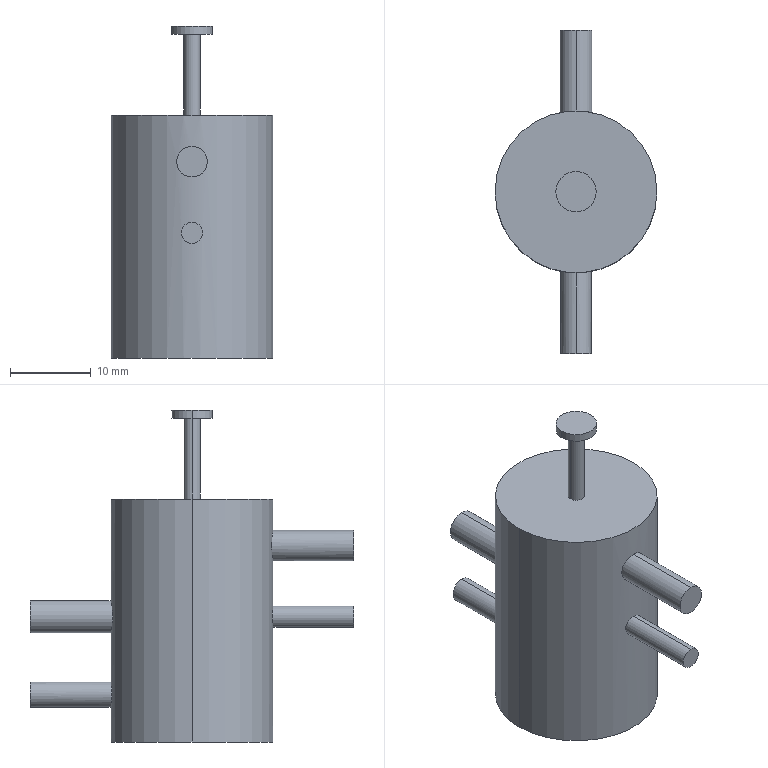Part | SolidWorks | features BaseBody 1 | 1 solid | 22 faces | box 20 x 40 x 41 mm | volume 9841 mm3 | cylinder 14 | plane 8 | commonest cylinder face diameters 2 x2 2.618 x2 3.076 x2 3.768 x2 3.973 x2 5 x2
STEP:
#1=CARTESIAN_POINT('',(0.,-20.,26.133));
#2=VERTEX_POINT('',#1);
#3=CARTESIAN_POINT('',(0.,-20.,22.365));
#4=VERTEX_POINT('',#3);
#5=CARTESIAN_POINT('',(0.,-20.,24.249));
#6=DIRECTION('',(0.,1.,0.));
#7=DIRECTION('',(0.,0.,1.));
#8=AXIS2_PLACEMENT_3D('',#5,#6,#7);
#9=CIRCLE('',#8,1.884);
#10=EDGE_CURVE('',#2,#4,#9,.T.);
#11=ORIENTED_EDGE('',*,*,#10,.T.);
#12=CARTESIAN_POINT('',(0.,-10.,22.365));
#13=VERTEX_POINT('',#12);
#14=CARTESIAN_POINT('',(0.,-20.,22.365));
#15=DIRECTION('',(0.,1.,0.));
#16=VECTOR('',#15,1000.);
#17=LINE('',#14,#16);
#18=EDGE_CURVE('',#4,#13,#17,.T.);
#19=ORIENTED_EDGE('',*,*,#18,.T.);
#20=CARTESIAN_POINT('',(0.,-10.,26.133));
#21=VERTEX_POINT('',#20);
#22=CARTESIAN_POINT('',(0.,-10.,26.133));
#23=CARTESIAN_POINT('',(0.1248,-10.,26.133));
#24=CARTESIAN_POINT('',(0.2474,-9.998,26.12));
#25=CARTESIAN_POINT('',(0.4886,-9.989,26.072));
#26=CARTESIAN_POINT('',(0.6084,-9.982,26.036));
#27=CARTESIAN_POINT('',(0.8364,-9.966,25.941));
#28=CARTESIAN_POINT('',(0.9445,-9.956,25.883));
#29=CARTESIAN_POINT('',(1.149,-9.934,25.747));
#30=CARTESIAN_POINT('',(1.246,-9.922,25.667));
#31=CARTESIAN_POINT('',(1.506,-9.888,25.407));
#32=CARTESIAN_POINT('',(1.646,-9.864,25.197));
#33=CARTESIAN_POINT('',(1.834,-9.831,24.744));
#34=CARTESIAN_POINT('',(1.884,-9.821,24.496));
#35=CARTESIAN_POINT('',(1.884,-9.821,24.126));
#36=CARTESIAN_POINT('',(1.872,-9.823,24.001));
#37=CARTESIAN_POINT('',(1.823,-9.832,23.759));
#38=CARTESIAN_POINT('',(1.788,-9.839,23.642));
#39=CARTESIAN_POINT('',(1.646,-9.864,23.299));
#40=CARTESIAN_POINT('',(1.507,-9.887,23.092));
#41=CARTESIAN_POINT('',(1.244,-9.923,22.829));
#42=CARTESIAN_POINT('',(1.15,-9.934,22.751));
#43=CARTESIAN_POINT('',(0.9458,-9.956,22.615));
#44=CARTESIAN_POINT('',(0.8355,-9.966,22.556));
#45=CARTESIAN_POINT('',(0.6077,-9.982,22.461));
#46=CARTESIAN_POINT('',(0.4902,-9.989,22.426));
#47=CARTESIAN_POINT('',(0.2481,-9.998,22.377));
#48=CARTESIAN_POINT('',(0.1231,-10.,22.365));
#49=CARTESIAN_POINT('',(0.,-10.,22.365));
#50=B_SPLINE_CURVE_WITH_KNOTS('',3,(#22,#23,#24,#25,#26,#27,#28,#29,#30,#31,#32,#33,#34,#35,#36,#37,#38,#39,#40,#41,#42,#43,#44,#45,#46,#47,#48,#49),.UNSPECIFIED.,.F.,.F.,(4,2,2,2,2,2,2,2,2,2,2,2,2,4),(0.,0.0003689,0.0007379,0.001107,0.001476,0.002214,0.002952,0.003321,0.003689,0.004427,0.004796,0.005165,0.005534,0.005903),.UNSPECIFIED.);
#51=EDGE_CURVE('',#21,#13,#50,.T.);
#52=ORIENTED_EDGE('',*,*,#51,.F.);
#53=CARTESIAN_POINT('',(0.,-20.,26.133));
#54=DIRECTION('',(0.,1.,0.));
#55=VECTOR('',#54,1000.);
#56=LINE('',#53,#55);
#57=EDGE_CURVE('',#2,#21,#56,.T.);
#58=ORIENTED_EDGE('',*,*,#57,.F.);
#59=EDGE_LOOP('',(#11,#19,#52,#58));
#60=FACE_OUTER_BOUND('',#59,.T.);
#61=CARTESIAN_POINT('',(0.,-20.,24.249));
#62=DIRECTION('',(0.,1.,0.));
#63=DIRECTION('',(0.,0.,1.));
#64=AXIS2_PLACEMENT_3D('',#61,#62,#63);
#65=CYLINDRICAL_SURFACE('',#64,1.884);
#66=ADVANCED_FACE('',(#60),#65,.T.);
#67=CARTESIAN_POINT('',(0.,-20.,16.779));
#68=VERTEX_POINT('',#67);
#69=CARTESIAN_POINT('',(0.,-20.,14.161));
#70=VERTEX_POINT('',#69);
#71=CARTESIAN_POINT('',(0.,-20.,15.47));
#72=DIRECTION('',(0.,1.,0.));
#73=DIRECTION('',(0.,0.,1.));
#74=AXIS2_PLACEMENT_3D('',#71,#72,#73);
#75=CIRCLE('',#74,1.309);
#76=EDGE_CURVE('',#68,#70,#75,.T.);
#77=ORIENTED_EDGE('',*,*,#76,.T.);
#78=CARTESIAN_POINT('',(0.,-10.,14.161));
#79=VERTEX_POINT('',#78);
#80=CARTESIAN_POINT('',(0.,-20.,14.161));
#81=DIRECTION('',(0.,1.,0.));
#82=VECTOR('',#81,1000.);
#83=LINE('',#80,#82);
#84=EDGE_CURVE('',#70,#79,#83,.T.);
#85=ORIENTED_EDGE('',*,*,#84,.T.);
#86=CARTESIAN_POINT('',(0.,-10.,16.779));
#87=VERTEX_POINT('',#86);
#88=CARTESIAN_POINT('',(0.,-10.,16.779));
#89=CARTESIAN_POINT('',(0.1732,-10.,16.779));
#90=CARTESIAN_POINT('',(0.3431,-9.995,16.744));
#91=CARTESIAN_POINT('',(0.5808,-9.983,16.646));
#92=CARTESIAN_POINT('',(0.656,-9.979,16.606));
#93=CARTESIAN_POINT('',(0.7982,-9.968,16.511));
#94=CARTESIAN_POINT('',(0.8655,-9.963,16.455));
#95=CARTESIAN_POINT('',(1.046,-9.946,16.274));
#96=CARTESIAN_POINT('',(1.144,-9.935,16.128));
#97=CARTESIAN_POINT('',(1.274,-9.919,15.813));
#98=CARTESIAN_POINT('',(1.309,-9.914,15.641));
#99=CARTESIAN_POINT('',(1.309,-9.914,15.385));
#100=CARTESIAN_POINT('',(1.3,-9.915,15.298));
#101=CARTESIAN_POINT('',(1.267,-9.919,15.13));
#102=CARTESIAN_POINT('',(1.242,-9.923,15.048));
#103=CARTESIAN_POINT('',(1.144,-9.935,14.81));
#104=CARTESIAN_POINT('',(1.048,-9.946,14.666));
#105=CARTESIAN_POINT('',(0.8036,-9.968,14.422));
#106=CARTESIAN_POINT('',(0.6596,-9.979,14.326));
#107=CARTESIAN_POINT('',(0.4219,-9.991,14.227));
#108=CARTESIAN_POINT('',(0.3402,-9.995,14.203));
#109=CARTESIAN_POINT('',(0.1723,-9.999,14.169));
#110=CARTESIAN_POINT('',(0.08548,-10.,14.161));
#111=CARTESIAN_POINT('',(0.,-10.,14.161));
#112=B_SPLINE_CURVE_WITH_KNOTS('',3,(#88,#89,#90,#91,#92,#93,#94,#95,#96,#97,#98,#99,#100,#101,#102,#103,#104,#105,#106,#107,#108,#109,#110,#111),.UNSPECIFIED.,.F.,.F.,(4,2,2,2,2,2,2,2,2,2,2,4),(0.,0.0005121,0.0007682,0.001024,0.001536,0.002048,0.002304,0.002561,0.003073,0.003585,0.003841,0.004097),.UNSPECIFIED.);
#113=EDGE_CURVE('',#87,#79,#112,.T.);
#114=ORIENTED_EDGE('',*,*,#113,.F.);
#115=CARTESIAN_POINT('',(0.,-20.,16.779));
#116=DIRECTION('',(0.,1.,0.));
#117=VECTOR('',#116,1000.);
#118=LINE('',#115,#117);
#119=EDGE_CURVE('',#68,#87,#118,.T.);
#120=ORIENTED_EDGE('',*,*,#119,.F.);
#121=EDGE_LOOP('',(#77,#85,#114,#120));
#122=FACE_OUTER_BOUND('',#121,.T.);
#123=CARTESIAN_POINT('',(0.,-20.,15.47));
#124=DIRECTION('',(0.,1.,0.));
#125=DIRECTION('',(0.,0.,1.));
#126=AXIS2_PLACEMENT_3D('',#123,#124,#125);
#127=CYLINDRICAL_SURFACE('',#126,1.309);
#128=ADVANCED_FACE('',(#122),#127,.T.);
#129=CARTESIAN_POINT('',(0.,20.,17.456));
#130=VERTEX_POINT('',#129);
#131=CARTESIAN_POINT('',(0.,20.,13.483));
#132=VERTEX_POINT('',#131);
#133=CARTESIAN_POINT('',(0.,20.,15.47));
#134=DIRECTION('',(0.,1.,0.));
#135=DIRECTION('',(0.,0.,1.));
#136=AXIS2_PLACEMENT_3D('',#133,#134,#135);
#137=CIRCLE('',#136,1.987);
#138=EDGE_CURVE('',#130,#132,#137,.T.);
#139=ORIENTED_EDGE('',*,*,#138,.F.);
#140=CARTESIAN_POINT('',(0.,10.,17.456));
#141=VERTEX_POINT('',#140);
#142=CARTESIAN_POINT('',(0.,20.,17.456));
#143=DIRECTION('',(0.,-1.,0.));
#144=VECTOR('',#143,1000.);
#145=LINE('',#142,#144);
#146=EDGE_CURVE('',#130,#141,#145,.T.);
#147=ORIENTED_EDGE('',*,*,#146,.T.);
#148=CARTESIAN_POINT('',(0.,10.,13.483));
#149=VERTEX_POINT('',#148);
#150=CARTESIAN_POINT('',(0.,10.,17.456));
#151=CARTESIAN_POINT('',(0.2596,10.,17.456));
#152=CARTESIAN_POINT('',(0.5216,9.989,17.404));
#153=CARTESIAN_POINT('',(0.8803,9.962,17.255));
#154=CARTESIAN_POINT('',(0.9963,9.951,17.193));
#155=CARTESIAN_POINT('',(1.213,9.927,17.049));
#156=CARTESIAN_POINT('',(1.312,9.914,16.967));
#157=CARTESIAN_POINT('',(1.496,9.888,16.784));
#158=CARTESIAN_POINT('',(1.579,9.875,16.682));
#159=CARTESIAN_POINT('',(1.723,9.851,16.467));
#160=CARTESIAN_POINT('',(1.784,9.84,16.353));
#161=CARTESIAN_POINT('',(1.935,9.812,15.991));
#162=CARTESIAN_POINT('',(1.986,9.801,15.733));
#163=CARTESIAN_POINT('',(1.987,9.801,15.339));
#164=CARTESIAN_POINT('',(1.974,9.803,15.21));
#165=CARTESIAN_POINT('',(1.923,9.813,14.956));
#166=CARTESIAN_POINT('',(1.885,9.821,14.829));
#167=CARTESIAN_POINT('',(1.785,9.839,14.589));
#168=CARTESIAN_POINT('',(1.725,9.85,14.475));
#169=CARTESIAN_POINT('',(1.58,9.875,14.259));
#170=CARTESIAN_POINT('',(1.497,9.888,14.157));
#171=CARTESIAN_POINT('',(1.223,9.927,13.883));
#172=CARTESIAN_POINT('',(1.002,9.953,13.735));
#173=CARTESIAN_POINT('',(0.6438,9.98,13.586));
#174=CARTESIAN_POINT('',(0.5178,9.987,13.547));
#175=CARTESIAN_POINT('',(0.2614,9.997,13.496));
#176=CARTESIAN_POINT('',(0.1316,10.,13.483));
#177=CARTESIAN_POINT('',(0.,10.,13.483));
#178=B_SPLINE_CURVE_WITH_KNOTS('',3,(#150,#151,#152,#153,#154,#155,#156,#157,#158,#159,#160,#161,#162,#163,#164,#165,#166,#167,#168,#169,#170,#171,#172,#173,#174,#175,#176,#177),.UNSPECIFIED.,.F.,.F.,(4,2,2,2,2,2,2,2,2,2,2,2,2,4),(0.006226,0.007004,0.007393,0.007783,0.008172,0.008561,0.009339,0.009728,0.01012,0.01051,0.01089,0.01167,0.01206,0.01245),.UNSPECIFIED.);
#179=EDGE_CURVE('',#141,#149,#178,.T.);
#180=ORIENTED_EDGE('',*,*,#179,.T.);
#181=CARTESIAN_POINT('',(0.,20.,13.483));
#182=DIRECTION('',(0.,-1.,0.));
#183=VECTOR('',#182,1000.);
#184=LINE('',#181,#183);
#185=EDGE_CURVE('',#132,#149,#184,.T.);
#186=ORIENTED_EDGE('',*,*,#185,.F.);
#187=EDGE_LOOP('',(#139,#147,#180,#186));
#188=FACE_OUTER_BOUND('',#187,.T.);
#189=CARTESIAN_POINT('',(0.,20.,15.47));
#190=DIRECTION('',(0.,-1.,0.));
#191=DIRECTION('',(0.,0.,-1.));
#192=AXIS2_PLACEMENT_3D('',#189,#190,#191);
#193=CYLINDRICAL_SURFACE('',#192,1.987);
#194=ADVANCED_FACE('',(#188),#193,.T.);
#195=CARTESIAN_POINT('',(0.,20.,7.395));
#196=VERTEX_POINT('',#195);
#197=CARTESIAN_POINT('',(0.,20.,4.319));
#198=VERTEX_POINT('',#197);
#199=CARTESIAN_POINT('',(0.,20.,5.857));
#200=DIRECTION('',(0.,1.,0.));
#201=DIRECTION('',(0.,0.,1.));
#202=AXIS2_PLACEMENT_3D('',#199,#200,#201);
#203=CIRCLE('',#202,1.538);
#204=EDGE_CURVE('',#196,#198,#203,.T.);
#205=ORIENTED_EDGE('',*,*,#204,.F.);
#206=CARTESIAN_POINT('',(0.,10.,7.395));
#207=VERTEX_POINT('',#206);
#208=CARTESIAN_POINT('',(0.,20.,7.395));
#209=DIRECTION('',(0.,-1.,0.));
#210=VECTOR('',#209,1000.);
#211=LINE('',#208,#210);
#212=EDGE_CURVE('',#196,#207,#211,.T.);
#213=ORIENTED_EDGE('',*,*,#212,.T.);
#214=CARTESIAN_POINT('',(0.,10.,4.319));
#215=VERTEX_POINT('',#214);
#216=CARTESIAN_POINT('',(0.,10.,7.395));
#217=CARTESIAN_POINT('',(0.2009,10.,7.395));
#218=CARTESIAN_POINT('',(0.4035,9.994,7.355));
#219=CARTESIAN_POINT('',(0.7737,9.972,7.201));
#220=CARTESIAN_POINT('',(0.945,9.956,7.087));
#221=CARTESIAN_POINT('',(1.158,9.933,6.875));
#222=CARTESIAN_POINT('',(1.223,9.925,6.796));
#223=CARTESIAN_POINT('',(1.334,9.911,6.629));
#224=CARTESIAN_POINT('',(1.381,9.904,6.541));
#225=CARTESIAN_POINT('',(1.498,9.888,6.261));
#226=CARTESIAN_POINT('',(1.538,9.881,6.061));
#227=CARTESIAN_POINT('',(1.538,9.881,5.757));
#228=CARTESIAN_POINT('',(1.528,9.883,5.657));
#229=CARTESIAN_POINT('',(1.489,9.889,5.46));
#230=CARTESIAN_POINT('',(1.459,9.893,5.362));
#231=CARTESIAN_POINT('',(1.382,9.904,5.176));
#232=CARTESIAN_POINT('',(1.335,9.911,5.088));
#233=CARTESIAN_POINT('',(1.224,9.925,4.92));
#234=CARTESIAN_POINT('',(1.159,9.933,4.841));
#235=CARTESIAN_POINT('',(0.9468,9.956,4.629));
#236=CARTESIAN_POINT('',(0.7755,9.972,4.514));
#237=CARTESIAN_POINT('',(0.4057,9.993,4.36));
#238=CARTESIAN_POINT('',(0.2035,10.,4.319));
#239=CARTESIAN_POINT('',(0.,10.,4.319));
#240=B_SPLINE_CURVE_WITH_KNOTS('',3,(#216,#217,#218,#219,#220,#221,#222,#223,#224,#225,#226,#227,#228,#229,#230,#231,#232,#233,#234,#235,#236,#237,#238,#239),.UNSPECIFIED.,.F.,.F.,(4,2,2,2,2,2,2,2,2,2,2,4),(0.004816,0.005417,0.006019,0.00632,0.006621,0.007223,0.007524,0.007825,0.008125,0.008426,0.009028,0.00963),.UNSPECIFIED.);
#241=EDGE_CURVE('',#207,#215,#240,.T.);
#242=ORIENTED_EDGE('',*,*,#241,.T.);
#243=CARTESIAN_POINT('',(0.,20.,4.319));
#244=DIRECTION('',(0.,-1.,0.));
#245=VECTOR('',#244,1000.);
#246=LINE('',#243,#245);
#247=EDGE_CURVE('',#198,#215,#246,.T.);
#248=ORIENTED_EDGE('',*,*,#247,.F.);
#249=EDGE_LOOP('',(#205,#213,#242,#248));
#250=FACE_OUTER_BOUND('',#249,.T.);
#251=CARTESIAN_POINT('',(0.,20.,5.857));
#252=DIRECTION('',(0.,-1.,0.));
#253=DIRECTION('',(0.,0.,-1.));
#254=AXIS2_PLACEMENT_3D('',#251,#252,#253);
#255=CYLINDRICAL_SURFACE('',#254,1.538);
#256=ADVANCED_FACE('',(#250),#255,.T.);
#257=CARTESIAN_POINT('',(2.5,0.,41.));
#258=VERTEX_POINT('',#257);
#259=CARTESIAN_POINT('',(-2.5,0.,41.));
#260=VERTEX_POINT('',#259);
#261=CARTESIAN_POINT('',(0.,0.,41.));
#262=DIRECTION('',(0.,0.,1.));
#263=DIRECTION('',(1.,0.,0.));
#264=AXIS2_PLACEMENT_3D('',#261,#262,#263);
#265=CIRCLE('',#264,2.5);
#266=EDGE_CURVE('',#258,#260,#265,.T.);
#267=ORIENTED_EDGE('',*,*,#266,.F.);
#268=CARTESIAN_POINT('',(2.5,0.,40.));
#269=VERTEX_POINT('',#268);
#270=CARTESIAN_POINT('',(2.5,0.,41.));
#271=DIRECTION('',(0.,0.,-1.));
#272=VECTOR('',#271,1000.);
#273=LINE('',#270,#272);
#274=EDGE_CURVE('',#258,#269,#273,.T.);
#275=ORIENTED_EDGE('',*,*,#274,.T.);
#276=CARTESIAN_POINT('',(-2.5,0.,40.));
#277=VERTEX_POINT('',#276);
#278=CARTESIAN_POINT('',(0.,0.,40.));
#279=DIRECTION('',(0.,0.,1.));
#280=DIRECTION('',(1.,0.,0.));
#281=AXIS2_PLACEMENT_3D('',#278,#279,#280);
#282=CIRCLE('',#281,2.5);
#283=EDGE_CURVE('',#269,#277,#282,.T.);
#284=ORIENTED_EDGE('',*,*,#283,.T.);
#285=CARTESIAN_POINT('',(-2.5,0.,41.));
#286=DIRECTION('',(0.,0.,-1.));
#287=VECTOR('',#286,1000.);
#288=LINE('',#285,#287);
#289=EDGE_CURVE('',#260,#277,#288,.T.);
#290=ORIENTED_EDGE('',*,*,#289,.F.);
#291=EDGE_LOOP('',(#267,#275,#284,#290));
#292=FACE_OUTER_BOUND('',#291,.T.);
#293=CARTESIAN_POINT('',(0.,0.,41.));
#294=DIRECTION('',(0.,0.,-1.));
#295=DIRECTION('',(-1.,0.,0.));
#296=AXIS2_PLACEMENT_3D('',#293,#294,#295);
#297=CYLINDRICAL_SURFACE('',#296,2.5);
#298=ADVANCED_FACE('',(#292),#297,.T.);
#299=CARTESIAN_POINT('',(1.,0.,40.));
#300=VERTEX_POINT('',#299);
#301=CARTESIAN_POINT('',(-1.,0.,40.));
#302=VERTEX_POINT('',#301);
#303=CARTESIAN_POINT('',(0.,0.,40.));
#304=DIRECTION('',(0.,0.,1.));
#305=DIRECTION('',(1.,0.,0.));
#306=AXIS2_PLACEMENT_3D('',#303,#304,#305);
#307=CIRCLE('',#306,1.);
#308=EDGE_CURVE('',#300,#302,#307,.T.);
#309=ORIENTED_EDGE('',*,*,#308,.F.);
#310=CARTESIAN_POINT('',(1.,0.,30.));
#311=VERTEX_POINT('',#310);
#312=CARTESIAN_POINT('',(1.,0.,40.));
#313=DIRECTION('',(0.,0.,-1.));
#314=VECTOR('',#313,1000.);
#315=LINE('',#312,#314);
#316=EDGE_CURVE('',#300,#311,#315,.T.);
#317=ORIENTED_EDGE('',*,*,#316,.T.);
#318=CARTESIAN_POINT('',(-1.,0.,30.));
#319=VERTEX_POINT('',#318);
#320=CARTESIAN_POINT('',(0.,0.,30.));
#321=DIRECTION('',(0.,0.,1.));
#322=DIRECTION('',(1.,0.,0.));
#323=AXIS2_PLACEMENT_3D('',#320,#321,#322);
#324=CIRCLE('',#323,1.);
#325=EDGE_CURVE('',#311,#319,#324,.T.);
#326=ORIENTED_EDGE('',*,*,#325,.T.);
#327=CARTESIAN_POINT('',(-1.,0.,40.));
#328=DIRECTION('',(0.,0.,-1.));
#329=VECTOR('',#328,1000.);
#330=LINE('',#327,#329);
#331=EDGE_CURVE('',#302,#319,#330,.T.);
#332=ORIENTED_EDGE('',*,*,#331,.F.);
#333=EDGE_LOOP('',(#309,#317,#326,#332));
#334=FACE_OUTER_BOUND('',#333,.T.);
#335=CARTESIAN_POINT('',(0.,0.,40.));
#336=DIRECTION('',(0.,0.,-1.));
#337=DIRECTION('',(-1.,0.,0.));
#338=AXIS2_PLACEMENT_3D('',#335,#336,#337);
#339=CYLINDRICAL_SURFACE('',#338,1.);
#340=ADVANCED_FACE('',(#334),#339,.T.);
#341=CARTESIAN_POINT('',(0.,10.,13.483));
#342=CARTESIAN_POINT('',(-0.1316,10.,13.483));
#343=CARTESIAN_POINT('',(-0.261,9.997,13.496));
#344=CARTESIAN_POINT('',(-0.5153,9.988,13.547));
#345=CARTESIAN_POINT('',(-0.6417,9.98,13.585));
#346=CARTESIAN_POINT('',(-0.8821,9.962,13.685));
#347=CARTESIAN_POINT('',(-0.9961,9.951,13.746));
#348=CARTESIAN_POINT('',(-1.212,9.927,13.89));
#349=CARTESIAN_POINT('',(-1.314,9.914,13.974));
#350=CARTESIAN_POINT('',(-1.588,9.875,14.248));
#351=CARTESIAN_POINT('',(-1.736,9.849,14.469));
#352=CARTESIAN_POINT('',(-1.934,9.812,14.947));
#353=CARTESIAN_POINT('',(-1.986,9.801,15.209));
#354=CARTESIAN_POINT('',(-1.987,9.801,15.599));
#355=CARTESIAN_POINT('',(-1.974,9.803,15.731));
#356=CARTESIAN_POINT('',(-1.923,9.813,15.986));
#357=CARTESIAN_POINT('',(-1.885,9.821,16.11));
#358=CARTESIAN_POINT('',(-1.735,9.849,16.471));
#359=CARTESIAN_POINT('',(-1.589,9.875,16.69));
#360=CARTESIAN_POINT('',(-1.312,9.914,16.967));
#361=CARTESIAN_POINT('',(-1.212,9.927,17.049));
#362=CARTESIAN_POINT('',(-0.9974,9.951,17.192));
#363=CARTESIAN_POINT('',(-0.881,9.962,17.255));
#364=CARTESIAN_POINT('',(-0.6409,9.98,17.354));
#365=CARTESIAN_POINT('',(-0.517,9.987,17.392));
#366=CARTESIAN_POINT('',(-0.2617,9.997,17.443));
#367=CARTESIAN_POINT('',(-0.1298,10.,17.456));
#368=CARTESIAN_POINT('',(0.,10.,17.456));
#369=B_SPLINE_CURVE_WITH_KNOTS('',3,(#341,#342,#343,#344,#345,#346,#347,#348,#349,#350,#351,#352,#353,#354,#355,#356,#357,#358,#359,#360,#361,#362,#363,#364,#365,#366,#367,#368),.UNSPECIFIED.,.F.,.F.,(4,2,2,2,2,2,2,2,2,2,2,2,2,4),(0.,0.0003891,0.0007783,0.001167,0.001557,0.002335,0.003113,0.003502,0.003891,0.00467,0.005059,0.005448,0.005837,0.006226),.UNSPECIFIED.);
#370=EDGE_CURVE('',#149,#141,#369,.T.);
#371=ORIENTED_EDGE('',*,*,#370,.F.);
#372=ORIENTED_EDGE('',*,*,#179,.F.);
#373=EDGE_LOOP('',(#371,#372));
#374=FACE_BOUND('',#373,.T.);
#375=CARTESIAN_POINT('',(0.,10.,4.319));
#376=CARTESIAN_POINT('',(-0.1018,10.,4.319));
#377=CARTESIAN_POINT('',(-0.2018,9.998,4.329));
#378=CARTESIAN_POINT('',(-0.3986,9.993,4.368));
#379=CARTESIAN_POINT('',(-0.4964,9.988,4.398));
#380=CARTESIAN_POINT('',(-0.6826,9.977,4.475));
#381=CARTESIAN_POINT('',(-0.7709,9.971,4.523));
#382=CARTESIAN_POINT('',(-0.9379,9.956,4.634));
#383=CARTESIAN_POINT('',(-1.017,9.948,4.699));
#384=CARTESIAN_POINT('',(-1.229,9.925,4.912));
#385=CARTESIAN_POINT('',(-1.344,9.91,5.083));
#386=CARTESIAN_POINT('',(-1.497,9.888,5.453));
#387=CARTESIAN_POINT('',(-1.538,9.881,5.656));
#388=CARTESIAN_POINT('',(-1.538,9.881,5.957));
#389=CARTESIAN_POINT('',(-1.528,9.883,6.059));
#390=CARTESIAN_POINT('',(-1.489,9.889,6.257));
#391=CARTESIAN_POINT('',(-1.46,9.893,6.353));
#392=CARTESIAN_POINT('',(-1.344,9.91,6.632));
#393=CARTESIAN_POINT('',(-1.231,9.925,6.801));
#394=CARTESIAN_POINT('',(-1.016,9.949,7.016));
#395=CARTESIAN_POINT('',(-0.9384,9.956,7.08));
#396=CARTESIAN_POINT('',(-0.7719,9.971,7.191));
#397=CARTESIAN_POINT('',(-0.6819,9.977,7.239));
#398=CARTESIAN_POINT('',(-0.4958,9.988,7.317));
#399=CARTESIAN_POINT('',(-0.3999,9.992,7.346));
#400=CARTESIAN_POINT('',(-0.2025,9.998,7.385));
#401=CARTESIAN_POINT('',(-0.1005,10.,7.395));
#402=CARTESIAN_POINT('',(0.,10.,7.395));
#403=B_SPLINE_CURVE_WITH_KNOTS('',3,(#375,#376,#377,#378,#379,#380,#381,#382,#383,#384,#385,#386,#387,#388,#389,#390,#391,#392,#393,#394,#395,#396,#397,#398,#399,#400,#401,#402),.UNSPECIFIED.,.F.,.F.,(4,2,2,2,2,2,2,2,2,2,2,2,2,4),(0.,0.000301,0.0006019,0.0009029,0.001204,0.001806,0.002408,0.002709,0.00301,0.003612,0.003913,0.004214,0.004515,0.004816),.UNSPECIFIED.);
#404=EDGE_CURVE('',#215,#207,#403,.T.);
#405=ORIENTED_EDGE('',*,*,#404,.F.);
#406=ORIENTED_EDGE('',*,*,#241,.F.);
#407=EDGE_LOOP('',(#405,#406));
#408=FACE_BOUND('',#407,.T.);
#409=CARTESIAN_POINT('',(10.,0.,30.));
#410=VERTEX_POINT('',#409);
#411=CARTESIAN_POINT('',(-10.,0.,30.));
#412=VERTEX_POINT('',#411);
#413=CARTESIAN_POINT('',(0.,0.,30.));
#414=DIRECTION('',(0.,0.,1.));
#415=DIRECTION('',(1.,0.,0.));
#416=AXIS2_PLACEMENT_3D('',#413,#414,#415);
#417=CIRCLE('',#416,10.);
#418=EDGE_CURVE('',#410,#412,#417,.T.);
#419=ORIENTED_EDGE('',*,*,#418,.F.);
#420=CARTESIAN_POINT('',(10.,0.,0.));
#421=VERTEX_POINT('',#420);
#422=CARTESIAN_POINT('',(10.,0.,30.));
#423=DIRECTION('',(0.,0.,-1.));
#424=VECTOR('',#423,1000.);
#425=LINE('',#422,#424);
#426=EDGE_CURVE('',#410,#421,#425,.T.);
#427=ORIENTED_EDGE('',*,*,#426,.T.);
#428=CARTESIAN_POINT('',(-10.,0.,0.));
#429=VERTEX_POINT('',#428);
#430=CARTESIAN_POINT('',(0.,0.,0.));
#431=DIRECTION('',(0.,0.,1.));
#432=DIRECTION('',(1.,0.,0.));
#433=AXIS2_PLACEMENT_3D('',#430,#431,#432);
#434=CIRCLE('',#433,10.);
#435=EDGE_CURVE('',#421,#429,#434,.T.);
#436=ORIENTED_EDGE('',*,*,#435,.T.);
#437=CARTESIAN_POINT('',(-10.,0.,30.));
#438=DIRECTION('',(0.,0.,-1.));
#439=VECTOR('',#438,1000.);
#440=LINE('',#437,#439);
#441=EDGE_CURVE('',#412,#429,#440,.T.);
#442=ORIENTED_EDGE('',*,*,#441,.F.);
#443=EDGE_LOOP('',(#419,#427,#436,#442));
#444=FACE_OUTER_BOUND('',#443,.T.);
#445=CARTESIAN_POINT('',(0.,0.,30.));
#446=DIRECTION('',(0.,0.,-1.));
#447=DIRECTION('',(-1.,0.,0.));
#448=AXIS2_PLACEMENT_3D('',#445,#446,#447);
#449=CYLINDRICAL_SURFACE('',#448,10.);
#450=ADVANCED_FACE('',(#374,#408,#444),#449,.T.);
#451=ORIENTED_EDGE('',*,*,#426,.F.);
#452=CARTESIAN_POINT('',(0.,0.,30.));
#453=DIRECTION('',(0.,0.,1.));
#454=DIRECTION('',(1.,0.,0.));
#455=AXIS2_PLACEMENT_3D('',#452,#453,#454);
#456=CIRCLE('',#455,10.);
#457=EDGE_CURVE('',#412,#410,#456,.T.);
#458=ORIENTED_EDGE('',*,*,#457,.F.);
#459=ORIENTED_EDGE('',*,*,#441,.T.);
#460=CARTESIAN_POINT('',(0.,0.,0.));
#461=DIRECTION('',(0.,0.,1.));
#462=DIRECTION('',(1.,0.,0.));
#463=AXIS2_PLACEMENT_3D('',#460,#461,#462);
#464=CIRCLE('',#463,10.);
#465=EDGE_CURVE('',#429,#421,#464,.T.);
#466=ORIENTED_EDGE('',*,*,#465,.T.);
#467=EDGE_LOOP('',(#451,#458,#459,#466));
#468=FACE_OUTER_BOUND('',#467,.T.);
#469=ORIENTED_EDGE('',*,*,#51,.T.);
#470=CARTESIAN_POINT('',(0.,-10.,22.365));
#471=CARTESIAN_POINT('',(-0.2461,-10.,22.365));
#472=CARTESIAN_POINT('',(-0.4945,-9.99,22.414));
#473=CARTESIAN_POINT('',(-0.8347,-9.966,22.555));
#474=CARTESIAN_POINT('',(-0.9446,-9.956,22.614));
#475=CARTESIAN_POINT('',(-1.15,-9.934,22.751));
#476=CARTESIAN_POINT('',(-1.244,-9.923,22.829));
#477=CARTESIAN_POINT('',(-1.418,-9.899,23.003));
#478=CARTESIAN_POINT('',(-1.498,-9.887,23.099));
#479=CARTESIAN_POINT('',(-1.634,-9.866,23.303));
#480=CARTESIAN_POINT('',(-1.692,-9.856,23.411));
#481=CARTESIAN_POINT('',(-1.835,-9.831,23.754));
#482=CARTESIAN_POINT('',(-1.884,-9.821,23.999));
#483=CARTESIAN_POINT('',(-1.884,-9.821,24.372));
#484=CARTESIAN_POINT('',(-1.872,-9.823,24.495));
#485=CARTESIAN_POINT('',(-1.824,-9.832,24.736));
#486=CARTESIAN_POINT('',(-1.788,-9.839,24.856));
#487=CARTESIAN_POINT('',(-1.693,-9.856,25.084));
#488=CARTESIAN_POINT('',(-1.635,-9.866,25.192));
#489=CARTESIAN_POINT('',(-1.499,-9.887,25.397));
#490=CARTESIAN_POINT('',(-1.42,-9.899,25.493));
#491=CARTESIAN_POINT('',(-1.16,-9.934,25.753));
#492=CARTESIAN_POINT('',(-0.9503,-9.957,25.894));
#493=CARTESIAN_POINT('',(-0.6105,-9.982,26.035));
#494=CARTESIAN_POINT('',(-0.4911,-9.989,26.072));
#495=CARTESIAN_POINT('',(-0.2479,-9.998,26.12));
#496=CARTESIAN_POINT('',(-0.1247,-10.,26.133));
#497=CARTESIAN_POINT('',(0.,-10.,26.133));
#498=B_SPLINE_CURVE_WITH_KNOTS('',3,(#470,#471,#472,#473,#474,#475,#476,#477,#478,#479,#480,#481,#482,#483,#484,#485,#486,#487,#488,#489,#490,#491,#492,#493,#494,#495,#496,#497),.UNSPECIFIED.,.F.,.F.,(4,2,2,2,2,2,2,2,2,2,2,2,2,4),(0.005903,0.006641,0.00701,0.007379,0.007747,0.008116,0.008854,0.009223,0.009592,0.00996,0.01033,0.01107,0.01144,0.0118),.UNSPECIFIED.);
#499=EDGE_CURVE('',#13,#21,#498,.T.);
#500=ORIENTED_EDGE('',*,*,#499,.T.);
#501=EDGE_LOOP('',(#469,#500));
#502=FACE_BOUND('',#501,.T.);
#503=ORIENTED_EDGE('',*,*,#113,.T.);
#504=CARTESIAN_POINT('',(0.,-10.,14.161));
#505=CARTESIAN_POINT('',(-0.1709,-10.,14.161));
#506=CARTESIAN_POINT('',(-0.3433,-9.995,14.195));
#507=CARTESIAN_POINT('',(-0.6584,-9.98,14.325));
#508=CARTESIAN_POINT('',(-0.8042,-9.968,14.423));
#509=CARTESIAN_POINT('',(-0.9853,-9.952,14.604));
#510=CARTESIAN_POINT('',(-1.041,-9.946,14.671));
#511=CARTESIAN_POINT('',(-1.136,-9.935,14.813));
#512=CARTESIAN_POINT('',(-1.176,-9.931,14.888));
#513=CARTESIAN_POINT('',(-1.275,-9.919,15.126));
#514=CARTESIAN_POINT('',(-1.309,-9.914,15.296));
#515=CARTESIAN_POINT('',(-1.309,-9.914,15.642));
#516=CARTESIAN_POINT('',(-1.275,-9.919,15.812));
#517=CARTESIAN_POINT('',(-1.177,-9.931,16.049));
#518=CARTESIAN_POINT('',(-1.137,-9.935,16.125));
#519=CARTESIAN_POINT('',(-1.042,-9.946,16.267));
#520=CARTESIAN_POINT('',(-0.9865,-9.951,16.334));
#521=CARTESIAN_POINT('',(-0.8057,-9.968,16.515));
#522=CARTESIAN_POINT('',(-0.6599,-9.979,16.613));
#523=CARTESIAN_POINT('',(-0.3451,-9.995,16.744));
#524=CARTESIAN_POINT('',(-0.1731,-10.,16.779));
#525=CARTESIAN_POINT('',(0.,-10.,16.779));
#526=B_SPLINE_CURVE_WITH_KNOTS('',3,(#504,#505,#506,#507,#508,#509,#510,#511,#512,#513,#514,#515,#516,#517,#518,#519,#520,#521,#522,#523,#524,#525),.UNSPECIFIED.,.F.,.F.,(4,2,2,2,2,2,2,2,2,2,4),(0.004097,0.004609,0.005121,0.005377,0.005633,0.006145,0.006657,0.006913,0.007169,0.007681,0.008193),.UNSPECIFIED.);
#527=EDGE_CURVE('',#79,#87,#526,.T.);
#528=ORIENTED_EDGE('',*,*,#527,.T.);
#529=EDGE_LOOP('',(#503,#528));
#530=FACE_BOUND('',#529,.T.);
#531=CARTESIAN_POINT('',(0.,0.,30.));
#532=DIRECTION('',(0.,0.,-1.));
#533=DIRECTION('',(-1.,0.,0.));
#534=AXIS2_PLACEMENT_3D('',#531,#532,#533);
#535=CYLINDRICAL_SURFACE('',#534,10.);
#536=ADVANCED_FACE('',(#468,#502,#530),#535,.T.);
#537=CARTESIAN_POINT('',(0.,0.,30.));
#538=DIRECTION('',(0.,0.,1.));
#539=DIRECTION('',(1.,0.,0.));
#540=AXIS2_PLACEMENT_3D('',#537,#538,#539);
#541=CIRCLE('',#540,1.);
#542=EDGE_CURVE('',#319,#311,#541,.T.);
#543=ORIENTED_EDGE('',*,*,#542,.F.);
#544=ORIENTED_EDGE('',*,*,#325,.F.);
#545=EDGE_LOOP('',(#543,#544));
#546=FACE_BOUND('',#545,.T.);
#547=ORIENTED_EDGE('',*,*,#457,.T.);
#548=ORIENTED_EDGE('',*,*,#418,.T.);
#549=EDGE_LOOP('',(#547,#548));
#550=FACE_OUTER_BOUND('',#549,.T.);
#551=CARTESIAN_POINT('',(0.,0.,30.));
#552=DIRECTION('',(0.,0.,1.));
#553=DIRECTION('',(1.,0.,0.));
#554=AXIS2_PLACEMENT_3D('',#551,#552,#553);
#555=PLANE('',#554);
#556=ADVANCED_FACE('',(#546,#550),#555,.T.);
#557=ORIENTED_EDGE('',*,*,#465,.F.);
#558=ORIENTED_EDGE('',*,*,#435,.F.);
#559=EDGE_LOOP('',(#557,#558));
#560=FACE_OUTER_BOUND('',#559,.T.);
#561=CARTESIAN_POINT('',(0.,0.,0.));
#562=DIRECTION('',(0.,0.,1.));
#563=DIRECTION('',(1.,0.,0.));
#564=AXIS2_PLACEMENT_3D('',#561,#562,#563);
#565=PLANE('',#564);
#566=ADVANCED_FACE('',(#560),#565,.F.);
#567=ORIENTED_EDGE('',*,*,#316,.F.);
#568=CARTESIAN_POINT('',(0.,0.,40.));
#569=DIRECTION('',(0.,0.,1.));
#570=DIRECTION('',(1.,0.,0.));
#571=AXIS2_PLACEMENT_3D('',#568,#569,#570);
#572=CIRCLE('',#571,1.);
#573=EDGE_CURVE('',#302,#300,#572,.T.);
#574=ORIENTED_EDGE('',*,*,#573,.F.);
#575=ORIENTED_EDGE('',*,*,#331,.T.);
#576=ORIENTED_EDGE('',*,*,#542,.T.);
#577=EDGE_LOOP('',(#567,#574,#575,#576));
#578=FACE_OUTER_BOUND('',#577,.T.);
#579=CARTESIAN_POINT('',(0.,0.,40.));
#580=DIRECTION('',(0.,0.,-1.));
#581=DIRECTION('',(-1.,0.,0.));
#582=AXIS2_PLACEMENT_3D('',#579,#580,#581);
#583=CYLINDRICAL_SURFACE('',#582,1.);
#584=ADVANCED_FACE('',(#578),#583,.T.);
#585=ORIENTED_EDGE('',*,*,#274,.F.);
#586=CARTESIAN_POINT('',(0.,0.,41.));
#587=DIRECTION('',(0.,0.,1.));
#588=DIRECTION('',(1.,0.,0.));
#589=AXIS2_PLACEMENT_3D('',#586,#587,#588);
#590=CIRCLE('',#589,2.5);
#591=EDGE_CURVE('',#260,#258,#590,.T.);
#592=ORIENTED_EDGE('',*,*,#591,.F.);
#593=ORIENTED_EDGE('',*,*,#289,.T.);
#594=CARTESIAN_POINT('',(0.,0.,40.));
#595=DIRECTION('',(0.,0.,1.));
#596=DIRECTION('',(1.,0.,0.));
#597=AXIS2_PLACEMENT_3D('',#594,#595,#596);
#598=CIRCLE('',#597,2.5);
#599=EDGE_CURVE('',#277,#269,#598,.T.);
#600=ORIENTED_EDGE('',*,*,#599,.T.);
#601=EDGE_LOOP('',(#585,#592,#593,#600));
#602=FACE_OUTER_BOUND('',#601,.T.);
#603=CARTESIAN_POINT('',(0.,0.,41.));
#604=DIRECTION('',(0.,0.,-1.));
#605=DIRECTION('',(-1.,0.,0.));
#606=AXIS2_PLACEMENT_3D('',#603,#604,#605);
#607=CYLINDRICAL_SURFACE('',#606,2.5);
#608=ADVANCED_FACE('',(#602),#607,.T.);
#609=ORIENTED_EDGE('',*,*,#591,.T.);
#610=ORIENTED_EDGE('',*,*,#266,.T.);
#611=EDGE_LOOP('',(#609,#610));
#612=FACE_OUTER_BOUND('',#611,.T.);
#613=CARTESIAN_POINT('',(0.,0.,41.));
#614=DIRECTION('',(0.,0.,1.));
#615=DIRECTION('',(1.,0.,0.));
#616=AXIS2_PLACEMENT_3D('',#613,#614,#615);
#617=PLANE('',#616);
#618=ADVANCED_FACE('',(#612),#617,.T.);
#619=ORIENTED_EDGE('',*,*,#573,.T.);
#620=ORIENTED_EDGE('',*,*,#308,.T.);
#621=EDGE_LOOP('',(#619,#620));
#622=FACE_BOUND('',#621,.T.);
#623=ORIENTED_EDGE('',*,*,#599,.F.);
#624=ORIENTED_EDGE('',*,*,#283,.F.);
#625=EDGE_LOOP('',(#623,#624));
#626=FACE_OUTER_BOUND('',#625,.T.);
#627=CARTESIAN_POINT('',(0.,0.,40.));
#628=DIRECTION('',(0.,0.,1.));
#629=DIRECTION('',(1.,0.,0.));
#630=AXIS2_PLACEMENT_3D('',#627,#628,#629);
#631=PLANE('',#630);
#632=ADVANCED_FACE('',(#622,#626),#631,.F.);
#633=ORIENTED_EDGE('',*,*,#212,.F.);
#634=CARTESIAN_POINT('',(0.,20.,5.857));
#635=DIRECTION('',(0.,1.,0.));
#636=DIRECTION('',(0.,0.,1.));
#637=AXIS2_PLACEMENT_3D('',#634,#635,#636);
#638=CIRCLE('',#637,1.538);
#639=EDGE_CURVE('',#198,#196,#638,.T.);
#640=ORIENTED_EDGE('',*,*,#639,.F.);
#641=ORIENTED_EDGE('',*,*,#247,.T.);
#642=ORIENTED_EDGE('',*,*,#404,.T.);
#643=EDGE_LOOP('',(#633,#640,#641,#642));
#644=FACE_OUTER_BOUND('',#643,.T.);
#645=CARTESIAN_POINT('',(0.,20.,5.857));
#646=DIRECTION('',(0.,-1.,0.));
#647=DIRECTION('',(0.,0.,-1.));
#648=AXIS2_PLACEMENT_3D('',#645,#646,#647);
#649=CYLINDRICAL_SURFACE('',#648,1.538);
#650=ADVANCED_FACE('',(#644),#649,.T.);
#651=ORIENTED_EDGE('',*,*,#639,.T.);
#652=ORIENTED_EDGE('',*,*,#204,.T.);
#653=EDGE_LOOP('',(#651,#652));
#654=FACE_OUTER_BOUND('',#653,.T.);
#655=CARTESIAN_POINT('',(0.,20.,5.857));
#656=DIRECTION('',(0.,1.,0.));
#657=DIRECTION('',(0.,0.,1.));
#658=AXIS2_PLACEMENT_3D('',#655,#656,#657);
#659=PLANE('',#658);
#660=ADVANCED_FACE('',(#654),#659,.T.);
#661=ORIENTED_EDGE('',*,*,#146,.F.);
#662=CARTESIAN_POINT('',(0.,20.,15.47));
#663=DIRECTION('',(0.,1.,0.));
#664=DIRECTION('',(0.,0.,1.));
#665=AXIS2_PLACEMENT_3D('',#662,#663,#664);
#666=CIRCLE('',#665,1.987);
#667=EDGE_CURVE('',#132,#130,#666,.T.);
#668=ORIENTED_EDGE('',*,*,#667,.F.);
#669=ORIENTED_EDGE('',*,*,#185,.T.);
#670=ORIENTED_EDGE('',*,*,#370,.T.);
#671=EDGE_LOOP('',(#661,#668,#669,#670));
#672=FACE_OUTER_BOUND('',#671,.T.);
#673=CARTESIAN_POINT('',(0.,20.,15.47));
#674=DIRECTION('',(0.,-1.,0.));
#675=DIRECTION('',(0.,0.,-1.));
#676=AXIS2_PLACEMENT_3D('',#673,#674,#675);
#677=CYLINDRICAL_SURFACE('',#676,1.987);
#678=ADVANCED_FACE('',(#672),#677,.T.);
#679=ORIENTED_EDGE('',*,*,#667,.T.);
#680=ORIENTED_EDGE('',*,*,#138,.T.);
#681=EDGE_LOOP('',(#679,#680));
#682=FACE_OUTER_BOUND('',#681,.T.);
#683=CARTESIAN_POINT('',(0.,20.,15.47));
#684=DIRECTION('',(0.,1.,0.));
#685=DIRECTION('',(0.,0.,1.));
#686=AXIS2_PLACEMENT_3D('',#683,#684,#685);
#687=PLANE('',#686);
#688=ADVANCED_FACE('',(#682),#687,.T.);
#689=ORIENTED_EDGE('',*,*,#84,.F.);
#690=CARTESIAN_POINT('',(0.,-20.,15.47));
#691=DIRECTION('',(0.,1.,0.));
#692=DIRECTION('',(0.,0.,1.));
#693=AXIS2_PLACEMENT_3D('',#690,#691,#692);
#694=CIRCLE('',#693,1.309);
#695=EDGE_CURVE('',#70,#68,#694,.T.);
#696=ORIENTED_EDGE('',*,*,#695,.T.);
#697=ORIENTED_EDGE('',*,*,#119,.T.);
#698=ORIENTED_EDGE('',*,*,#527,.F.);
#699=EDGE_LOOP('',(#689,#696,#697,#698));
#700=FACE_OUTER_BOUND('',#699,.T.);
#701=CARTESIAN_POINT('',(0.,-20.,15.47));
#702=DIRECTION('',(0.,1.,0.));
#703=DIRECTION('',(0.,0.,1.));
#704=AXIS2_PLACEMENT_3D('',#701,#702,#703);
#705=CYLINDRICAL_SURFACE('',#704,1.309);
#706=ADVANCED_FACE('',(#700),#705,.T.);
#707=ORIENTED_EDGE('',*,*,#76,.F.);
#708=ORIENTED_EDGE('',*,*,#695,.F.);
#709=EDGE_LOOP('',(#707,#708));
#710=FACE_OUTER_BOUND('',#709,.T.);
#711=CARTESIAN_POINT('',(0.,-20.,15.47));
#712=DIRECTION('',(0.,1.,0.));
#713=DIRECTION('',(0.,0.,1.));
#714=AXIS2_PLACEMENT_3D('',#711,#712,#713);
#715=PLANE('',#714);
#716=ADVANCED_FACE('',(#710),#715,.F.);
#717=ORIENTED_EDGE('',*,*,#18,.F.);
#718=CARTESIAN_POINT('',(0.,-20.,24.249));
#719=DIRECTION('',(0.,1.,0.));
#720=DIRECTION('',(0.,0.,1.));
#721=AXIS2_PLACEMENT_3D('',#718,#719,#720);
#722=CIRCLE('',#721,1.884);
#723=EDGE_CURVE('',#4,#2,#722,.T.);
#724=ORIENTED_EDGE('',*,*,#723,.T.);
#725=ORIENTED_EDGE('',*,*,#57,.T.);
#726=ORIENTED_EDGE('',*,*,#499,.F.);
#727=EDGE_LOOP('',(#717,#724,#725,#726));
#728=FACE_OUTER_BOUND('',#727,.T.);
#729=CARTESIAN_POINT('',(0.,-20.,24.249));
#730=DIRECTION('',(0.,1.,0.));
#731=DIRECTION('',(0.,0.,1.));
#732=AXIS2_PLACEMENT_3D('',#729,#730,#731);
#733=CYLINDRICAL_SURFACE('',#732,1.884);
#734=ADVANCED_FACE('',(#728),#733,.T.);
#735=ORIENTED_EDGE('',*,*,#10,.F.);
#736=ORIENTED_EDGE('',*,*,#723,.F.);
#737=EDGE_LOOP('',(#735,#736));
#738=FACE_OUTER_BOUND('',#737,.T.);
#739=CARTESIAN_POINT('',(0.,-20.,24.249));
#740=DIRECTION('',(0.,1.,0.));
#741=DIRECTION('',(0.,0.,1.));
#742=AXIS2_PLACEMENT_3D('',#739,#740,#741);
#743=PLANE('',#742);
#744=ADVANCED_FACE('',(#738),#743,.F.);
#745=CLOSED_SHELL('',(#66,#128,#194,#256,#298,#340,#450,#536,#556,#566,#584,#608,#618,#632,#650,#660,#678,#688,#706,#716,#734,#744));
#746=MANIFOLD_SOLID_BREP('',#745);
#747=CARTESIAN_POINT('',(0.,0.,0.));
#748=DIRECTION('',(0.,0.,1.));
#749=DIRECTION('',(1.,0.,0.));
#750=AXIS2_PLACEMENT_3D('',#747,#748,#749);
#751=(LENGTH_UNIT()NAMED_UNIT(*)SI_UNIT(.MILLI.,.METRE.));
#752=UNCERTAINTY_MEASURE_WITH_UNIT(LENGTH_MEASURE(0.00001),#751,'','');
#753=(NAMED_UNIT(*)PLANE_ANGLE_UNIT()SI_UNIT($,.RADIAN.));
#754=(NAMED_UNIT(*)SI_UNIT($,.STERADIAN.)SOLID_ANGLE_UNIT());
#755=(GEOMETRIC_REPRESENTATION_CONTEXT(3)GLOBAL_UNCERTAINTY_ASSIGNED_CONTEXT((#752))GLOBAL_UNIT_ASSIGNED_CONTEXT((#751,#753,#754))REPRESENTATION_CONTEXT('',''));
#756=ADVANCED_BREP_SHAPE_REPRESENTATION('',(#746,#750),#755);